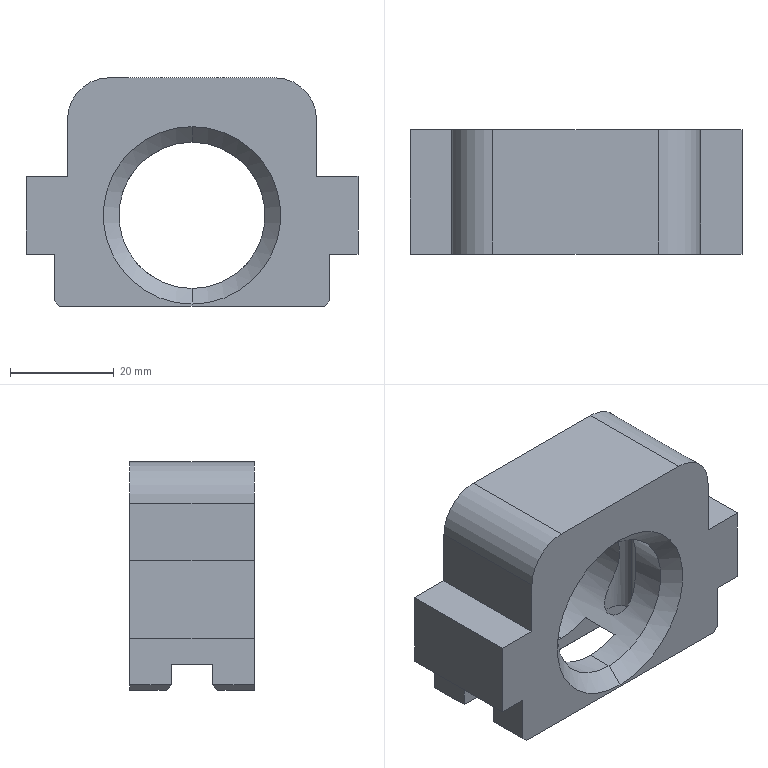Part | SolidWorks | features ICE 3, Chamfer 2, Extrusion 1 | 1 solid | 37 faces | box 64 x 24 x 44 mm | volume 38268 mm3 | plane 27 | cylinder 8 | cone 2 | commonest cylinder face diameters 6 x4 16 x2 28.2 x2
STEP:
#1=CARTESIAN_POINT('',(0.,3.,-12.4));
#2=VERTEX_POINT('',#1);
#3=CARTESIAN_POINT('',(0.,3.,-40.6));
#4=VERTEX_POINT('',#3);
#5=CARTESIAN_POINT('',(0.,3.,-26.5));
#6=DIRECTION('',(0.,-1.,0.));
#7=DIRECTION('',(0.,0.,1.));
#8=AXIS2_PLACEMENT_3D('',#5,#6,#7);
#9=CIRCLE('',#8,14.1);
#10=EDGE_CURVE('',#2,#4,#9,.T.);
#11=ORIENTED_EDGE('',*,*,#10,.F.);
#12=CARTESIAN_POINT('',(0.,0.,-9.4));
#13=VERTEX_POINT('',#12);
#14=CARTESIAN_POINT('',(0.,3.,-12.4));
#15=DIRECTION('',(0.,-0.7071,0.7071));
#16=VECTOR('',#15,1000.);
#17=LINE('',#14,#16);
#18=EDGE_CURVE('',#2,#13,#17,.T.);
#19=ORIENTED_EDGE('',*,*,#18,.T.);
#20=CARTESIAN_POINT('',(0.,0.,-43.6));
#21=VERTEX_POINT('',#20);
#22=CARTESIAN_POINT('',(0.,0.,-26.5));
#23=DIRECTION('',(0.,1.,0.));
#24=DIRECTION('',(0.,0.,1.));
#25=AXIS2_PLACEMENT_3D('',#22,#23,#24);
#26=CIRCLE('',#25,17.1);
#27=EDGE_CURVE('',#21,#13,#26,.T.);
#28=ORIENTED_EDGE('',*,*,#27,.F.);
#29=CARTESIAN_POINT('',(0.,3.,-40.6));
#30=DIRECTION('',(0.,-0.7071,-0.7071));
#31=VECTOR('',#30,1000.);
#32=LINE('',#29,#31);
#33=EDGE_CURVE('',#4,#21,#32,.T.);
#34=ORIENTED_EDGE('',*,*,#33,.F.);
#35=EDGE_LOOP('',(#11,#19,#28,#34));
#36=FACE_OUTER_BOUND('',#35,.T.);
#37=CARTESIAN_POINT('',(0.,3.,-26.5));
#38=DIRECTION('',(0.,-1.,0.));
#39=DIRECTION('',(0.,0.,-1.));
#40=AXIS2_PLACEMENT_3D('',#37,#38,#39);
#41=CONICAL_SURFACE('',#40,14.1,0.7854);
#42=ADVANCED_FACE('',(#36),#41,.F.);
#43=CARTESIAN_POINT('',(-9.,12.,-15.646));
#44=VERTEX_POINT('',#43);
#45=CARTESIAN_POINT('',(-9.,12.,-37.354));
#46=VERTEX_POINT('',#45);
#47=CARTESIAN_POINT('',(-9.,12.,-15.646));
#48=CARTESIAN_POINT('',(-9.,11.703,-15.646));
#49=CARTESIAN_POINT('',(-9.044,11.415,-15.682));
#50=CARTESIAN_POINT('',(-9.167,11.003,-15.787));
#51=CARTESIAN_POINT('',(-9.217,10.872,-15.829));
#52=CARTESIAN_POINT('',(-9.332,10.622,-15.93));
#53=CARTESIAN_POINT('',(-9.397,10.502,-15.988));
#54=CARTESIAN_POINT('',(-9.61,10.167,-16.181));
#55=CARTESIAN_POINT('',(-9.774,9.975,-16.335));
#56=CARTESIAN_POINT('',(-10.121,9.649,-16.68));
#57=CARTESIAN_POINT('',(-10.301,9.518,-16.868));
#58=CARTESIAN_POINT('',(-10.665,9.305,-17.273));
#59=CARTESIAN_POINT('',(-10.849,9.223,-17.49));
#60=CARTESIAN_POINT('',(-11.204,9.101,-17.935));
#61=CARTESIAN_POINT('',(-11.377,9.061,-18.165));
#62=CARTESIAN_POINT('',(-11.71,9.009,-18.64));
#63=CARTESIAN_POINT('',(-11.871,8.999,-18.886));
#64=CARTESIAN_POINT('',(-12.176,9.001,-19.384));
#65=CARTESIAN_POINT('',(-12.32,9.014,-19.636));
#66=CARTESIAN_POINT('',(-12.726,9.076,-20.402));
#67=CARTESIAN_POINT('',(-12.964,9.15,-20.925));
#68=CARTESIAN_POINT('',(-13.375,9.324,-22.));
#69=CARTESIAN_POINT('',(-13.548,9.425,-22.55));
#70=CARTESIAN_POINT('',(-13.823,9.612,-23.661));
#71=CARTESIAN_POINT('',(-13.927,9.699,-24.225));
#72=CARTESIAN_POINT('',(-14.067,9.823,-25.372));
#73=CARTESIAN_POINT('',(-14.101,9.859,-25.96));
#74=CARTESIAN_POINT('',(-14.098,9.856,-27.112));
#75=CARTESIAN_POINT('',(-14.062,9.819,-27.683));
#76=CARTESIAN_POINT('',(-13.92,9.693,-28.814));
#77=CARTESIAN_POINT('',(-13.816,9.606,-29.375));
#78=CARTESIAN_POINT('',(-13.396,9.324,-31.046));
#79=CARTESIAN_POINT('',(-12.988,9.114,-32.109));
#80=CARTESIAN_POINT('',(-12.307,9.013,-33.387));
#81=CARTESIAN_POINT('',(-12.161,9.,-33.641));
#82=CARTESIAN_POINT('',(-11.856,9.,-34.137));
#83=CARTESIAN_POINT('',(-11.696,9.011,-34.38));
#84=CARTESIAN_POINT('',(-11.362,9.064,-34.854));
#85=CARTESIAN_POINT('',(-11.187,9.106,-35.087));
#86=CARTESIAN_POINT('',(-10.833,9.23,-35.53));
#87=CARTESIAN_POINT('',(-10.653,9.311,-35.741));
#88=CARTESIAN_POINT('',(-10.293,9.524,-36.14));
#89=CARTESIAN_POINT('',(-10.11,9.658,-36.331));
#90=CARTESIAN_POINT('',(-9.852,9.902,-36.587));
#91=CARTESIAN_POINT('',(-9.769,9.99,-36.668));
#92=CARTESIAN_POINT('',(-9.61,10.183,-36.819));
#93=CARTESIAN_POINT('',(-9.533,10.288,-36.89));
#94=CARTESIAN_POINT('',(-9.322,10.622,-37.08));
#95=CARTESIAN_POINT('',(-9.207,10.869,-37.18));
#96=CARTESIAN_POINT('',(-9.043,11.419,-37.319));
#97=CARTESIAN_POINT('',(-9.,11.705,-37.354));
#98=CARTESIAN_POINT('',(-9.,12.,-37.354));
#99=B_SPLINE_CURVE_WITH_KNOTS('',3,(#47,#48,#49,#50,#51,#52,#53,#54,#55,#56,#57,#58,#59,#60,#61,#62,#63,#64,#65,#66,#67,#68,#69,#70,#71,#72,#73,#74,#75,#76,#77,#78,#79,#80,#81,#82,#83,#84,#85,#86,#87,#88,#89,#90,#91,#92,#93,#94,#95,#96,#97,#98),.UNSPECIFIED.,.F.,.F.,(4,2,2,2,2,2,2,2,2,2,2,2,2,2,2,2,2,2,2,2,2,2,2,2,2,4),(0.,0.0008757,0.001313,0.001751,0.002627,0.003503,0.004378,0.005254,0.00613,0.007005,0.008757,0.01051,0.01226,0.01401,0.01576,0.01751,0.02102,0.02189,0.02277,0.02364,0.02452,0.02539,0.02583,0.02627,0.02715,0.02802),.UNSPECIFIED.);
#100=EDGE_CURVE('',#44,#46,#99,.T.);
#101=ORIENTED_EDGE('',*,*,#100,.F.);
#102=CARTESIAN_POINT('',(-9.,12.,-37.354));
#103=CARTESIAN_POINT('',(-9.,12.295,-37.354));
#104=CARTESIAN_POINT('',(-9.044,12.585,-37.318));
#105=CARTESIAN_POINT('',(-9.167,12.997,-37.214));
#106=CARTESIAN_POINT('',(-9.217,13.128,-37.171));
#107=CARTESIAN_POINT('',(-9.331,13.377,-37.071));
#108=CARTESIAN_POINT('',(-9.397,13.497,-37.013));
#109=CARTESIAN_POINT('',(-9.609,13.832,-36.82));
#110=CARTESIAN_POINT('',(-9.773,14.024,-36.667));
#111=CARTESIAN_POINT('',(-10.119,14.349,-36.322));
#112=CARTESIAN_POINT('',(-10.298,14.48,-36.135));
#113=CARTESIAN_POINT('',(-10.662,14.693,-35.731));
#114=CARTESIAN_POINT('',(-10.846,14.775,-35.514));
#115=CARTESIAN_POINT('',(-11.2,14.897,-35.07));
#116=CARTESIAN_POINT('',(-11.372,14.938,-34.841));
#117=CARTESIAN_POINT('',(-11.705,14.99,-34.367));
#118=CARTESIAN_POINT('',(-11.867,15.001,-34.121));
#119=CARTESIAN_POINT('',(-12.171,14.999,-33.625));
#120=CARTESIAN_POINT('',(-12.315,14.987,-33.373));
#121=CARTESIAN_POINT('',(-12.721,14.925,-32.609));
#122=CARTESIAN_POINT('',(-12.959,14.851,-32.087));
#123=CARTESIAN_POINT('',(-13.37,14.678,-31.014));
#124=CARTESIAN_POINT('',(-13.543,14.578,-30.465));
#125=CARTESIAN_POINT('',(-13.819,14.392,-29.359));
#126=CARTESIAN_POINT('',(-13.923,14.305,-28.8));
#127=CARTESIAN_POINT('',(-14.029,14.211,-27.946));
#128=CARTESIAN_POINT('',(-14.055,14.186,-27.66));
#129=CARTESIAN_POINT('',(-14.091,14.151,-27.081));
#130=CARTESIAN_POINT('',(-14.1,14.142,-26.787));
#131=CARTESIAN_POINT('',(-14.1,14.143,-25.912));
#132=CARTESIAN_POINT('',(-14.064,14.18,-25.337));
#133=CARTESIAN_POINT('',(-13.923,14.304,-24.202));
#134=CARTESIAN_POINT('',(-13.819,14.391,-23.642));
#135=CARTESIAN_POINT('',(-13.542,14.579,-22.532));
#136=CARTESIAN_POINT('',(-13.369,14.679,-21.982));
#137=CARTESIAN_POINT('',(-12.959,14.851,-20.915));
#138=CARTESIAN_POINT('',(-12.723,14.924,-20.395));
#139=CARTESIAN_POINT('',(-12.318,14.986,-19.632));
#140=CARTESIAN_POINT('',(-12.175,14.999,-19.381));
#141=CARTESIAN_POINT('',(-11.87,15.001,-18.885));
#142=CARTESIAN_POINT('',(-11.709,14.991,-18.638));
#143=CARTESIAN_POINT('',(-11.374,14.939,-18.162));
#144=CARTESIAN_POINT('',(-11.201,14.898,-17.931));
#145=CARTESIAN_POINT('',(-10.844,14.775,-17.483));
#146=CARTESIAN_POINT('',(-10.661,14.693,-17.268));
#147=CARTESIAN_POINT('',(-10.299,14.48,-16.866));
#148=CARTESIAN_POINT('',(-10.119,14.35,-16.678));
#149=CARTESIAN_POINT('',(-9.771,14.022,-16.332));
#150=CARTESIAN_POINT('',(-9.61,13.832,-16.18));
#151=CARTESIAN_POINT('',(-9.397,13.497,-15.987));
#152=CARTESIAN_POINT('',(-9.331,13.377,-15.929));
#153=CARTESIAN_POINT('',(-9.217,13.129,-15.829));
#154=CARTESIAN_POINT('',(-9.168,12.999,-15.787));
#155=CARTESIAN_POINT('',(-9.086,12.727,-15.718));
#156=CARTESIAN_POINT('',(-9.054,12.584,-15.691));
#157=CARTESIAN_POINT('',(-9.011,12.295,-15.655));
#158=CARTESIAN_POINT('',(-9.,12.148,-15.646));
#159=CARTESIAN_POINT('',(-9.,12.,-15.646));
#160=B_SPLINE_CURVE_WITH_KNOTS('',3,(#102,#103,#104,#105,#106,#107,#108,#109,#110,#111,#112,#113,#114,#115,#116,#117,#118,#119,#120,#121,#122,#123,#124,#125,#126,#127,#128,#129,#130,#131,#132,#133,#134,#135,#136,#137,#138,#139,#140,#141,#142,#143,#144,#145,#146,#147,#148,#149,#150,#151,#152,#153,#154,#155,#156,#157,#158,#159),.UNSPECIFIED.,.F.,.F.,(4,2,2,2,2,2,2,2,2,2,2,2,2,2,2,2,2,2,2,2,2,2,2,2,2,2,2,2,4),(0.02802,0.0289,0.02933,0.02977,0.03065,0.03152,0.0324,0.03327,0.03415,0.03502,0.03677,0.03853,0.04028,0.04115,0.04203,0.04378,0.04553,0.04728,0.04903,0.04991,0.05078,0.05166,0.05253,0.05341,0.05428,0.05472,0.05516,0.05559,0.05603),.UNSPECIFIED.);
#161=EDGE_CURVE('',#46,#44,#160,.T.);
#162=ORIENTED_EDGE('',*,*,#161,.F.);
#163=EDGE_LOOP('',(#101,#162));
#164=FACE_BOUND('',#163,.T.);
#165=CARTESIAN_POINT('',(0.,24.,-40.6));
#166=VERTEX_POINT('',#165);
#167=CARTESIAN_POINT('',(0.,24.,-12.4));
#168=VERTEX_POINT('',#167);
#169=CARTESIAN_POINT('',(0.,24.,-26.5));
#170=DIRECTION('',(0.,1.,0.));
#171=DIRECTION('',(0.,0.,1.));
#172=AXIS2_PLACEMENT_3D('',#169,#170,#171);
#173=CIRCLE('',#172,14.1);
#174=EDGE_CURVE('',#166,#168,#173,.T.);
#175=ORIENTED_EDGE('',*,*,#174,.T.);
#176=CARTESIAN_POINT('',(0.,35.,-12.4));
#177=DIRECTION('',(0.,-1.,0.));
#178=VECTOR('',#177,1000.);
#179=LINE('',#176,#178);
#180=EDGE_CURVE('',#168,#2,#179,.T.);
#181=ORIENTED_EDGE('',*,*,#180,.T.);
#182=ORIENTED_EDGE('',*,*,#10,.T.);
#183=CARTESIAN_POINT('',(0.,8.,-40.6));
#184=VERTEX_POINT('',#183);
#185=CARTESIAN_POINT('',(0.,35.,-40.6));
#186=DIRECTION('',(0.,-1.,0.));
#187=VECTOR('',#186,1000.);
#188=LINE('',#185,#187);
#189=EDGE_CURVE('',#184,#4,#188,.T.);
#190=ORIENTED_EDGE('',*,*,#189,.F.);
#191=CARTESIAN_POINT('',(-6.524,8.,-39.));
#192=VERTEX_POINT('',#191);
#193=CARTESIAN_POINT('',(0.,8.,-26.5));
#194=DIRECTION('',(0.,-1.,0.));
#195=DIRECTION('',(0.,0.,-1.));
#196=AXIS2_PLACEMENT_3D('',#193,#194,#195);
#197=CIRCLE('',#196,14.1);
#198=EDGE_CURVE('',#192,#184,#197,.T.);
#199=ORIENTED_EDGE('',*,*,#198,.F.);
#200=CARTESIAN_POINT('',(-6.524,16.,-39.));
#201=VERTEX_POINT('',#200);
#202=CARTESIAN_POINT('',(-6.524,35.,-39.));
#203=DIRECTION('',(0.,-1.,0.));
#204=VECTOR('',#203,1000.);
#205=LINE('',#202,#204);
#206=EDGE_CURVE('',#201,#192,#205,.T.);
#207=ORIENTED_EDGE('',*,*,#206,.F.);
#208=CARTESIAN_POINT('',(0.,16.,-40.6));
#209=VERTEX_POINT('',#208);
#210=CARTESIAN_POINT('',(0.,16.,-26.5));
#211=DIRECTION('',(0.,1.,0.));
#212=DIRECTION('',(0.,0.,1.));
#213=AXIS2_PLACEMENT_3D('',#210,#211,#212);
#214=CIRCLE('',#213,14.1);
#215=EDGE_CURVE('',#209,#201,#214,.T.);
#216=ORIENTED_EDGE('',*,*,#215,.F.);
#217=CARTESIAN_POINT('',(0.,35.,-40.6));
#218=DIRECTION('',(0.,-1.,0.));
#219=VECTOR('',#218,1000.);
#220=LINE('',#217,#219);
#221=EDGE_CURVE('',#166,#209,#220,.T.);
#222=ORIENTED_EDGE('',*,*,#221,.F.);
#223=EDGE_LOOP('',(#175,#181,#182,#190,#199,#207,#216,#222));
#224=FACE_OUTER_BOUND('',#223,.T.);
#225=CARTESIAN_POINT('',(0.,35.,-26.5));
#226=DIRECTION('',(0.,-1.,0.));
#227=DIRECTION('',(0.,0.,-1.));
#228=AXIS2_PLACEMENT_3D('',#225,#226,#227);
#229=CYLINDRICAL_SURFACE('',#228,14.1);
#230=ADVANCED_FACE('',(#164,#224),#229,.F.);
#231=CARTESIAN_POINT('',(15.,12.,-4.));
#232=VERTEX_POINT('',#231);
#233=CARTESIAN_POINT('',(9.,12.,-4.));
#234=VERTEX_POINT('',#233);
#235=CARTESIAN_POINT('',(12.,12.,-4.));
#236=DIRECTION('',(0.,0.,-1.));
#237=DIRECTION('',(-1.,0.,0.));
#238=AXIS2_PLACEMENT_3D('',#235,#236,#237);
#239=CIRCLE('',#238,3.);
#240=EDGE_CURVE('',#232,#234,#239,.T.);
#241=ORIENTED_EDGE('',*,*,#240,.F.);
#242=CARTESIAN_POINT('',(15.,12.,-39.));
#243=VERTEX_POINT('',#242);
#244=CARTESIAN_POINT('',(15.,12.,-4.));
#245=DIRECTION('',(0.,0.,-1.));
#246=VECTOR('',#245,1000.);
#247=LINE('',#244,#246);
#248=EDGE_CURVE('',#232,#243,#247,.T.);
#249=ORIENTED_EDGE('',*,*,#248,.T.);
#250=CARTESIAN_POINT('',(9.,12.,-39.));
#251=VERTEX_POINT('',#250);
#252=CARTESIAN_POINT('',(12.,12.,-39.));
#253=DIRECTION('',(0.,0.,-1.));
#254=DIRECTION('',(-1.,0.,0.));
#255=AXIS2_PLACEMENT_3D('',#252,#253,#254);
#256=CIRCLE('',#255,3.);
#257=EDGE_CURVE('',#243,#251,#256,.T.);
#258=ORIENTED_EDGE('',*,*,#257,.T.);
#259=CARTESIAN_POINT('',(9.,12.,-37.354));
#260=VERTEX_POINT('',#259);
#261=CARTESIAN_POINT('',(9.,12.,-4.));
#262=DIRECTION('',(0.,0.,-1.));
#263=VECTOR('',#262,1000.);
#264=LINE('',#261,#263);
#265=EDGE_CURVE('',#260,#251,#264,.T.);
#266=ORIENTED_EDGE('',*,*,#265,.F.);
#267=CARTESIAN_POINT('',(9.,12.,-15.646));
#268=VERTEX_POINT('',#267);
#269=CARTESIAN_POINT('',(9.,12.,-37.354));
#270=CARTESIAN_POINT('',(9.,11.705,-37.354));
#271=CARTESIAN_POINT('',(9.044,11.415,-37.318));
#272=CARTESIAN_POINT('',(9.167,11.003,-37.214));
#273=CARTESIAN_POINT('',(9.217,10.872,-37.171));
#274=CARTESIAN_POINT('',(9.331,10.623,-37.071));
#275=CARTESIAN_POINT('',(9.397,10.503,-37.013));
#276=CARTESIAN_POINT('',(9.609,10.168,-36.82));
#277=CARTESIAN_POINT('',(9.773,9.976,-36.667));
#278=CARTESIAN_POINT('',(10.119,9.651,-36.322));
#279=CARTESIAN_POINT('',(10.298,9.52,-36.135));
#280=CARTESIAN_POINT('',(10.662,9.307,-35.731));
#281=CARTESIAN_POINT('',(10.846,9.225,-35.514));
#282=CARTESIAN_POINT('',(11.2,9.103,-35.07));
#283=CARTESIAN_POINT('',(11.372,9.062,-34.841));
#284=CARTESIAN_POINT('',(11.705,9.01,-34.367));
#285=CARTESIAN_POINT('',(11.867,8.999,-34.121));
#286=CARTESIAN_POINT('',(12.171,9.001,-33.625));
#287=CARTESIAN_POINT('',(12.315,9.013,-33.373));
#288=CARTESIAN_POINT('',(12.721,9.075,-32.609));
#289=CARTESIAN_POINT('',(12.959,9.149,-32.087));
#290=CARTESIAN_POINT('',(13.37,9.322,-31.014));
#291=CARTESIAN_POINT('',(13.543,9.422,-30.465));
#292=CARTESIAN_POINT('',(13.819,9.608,-29.359));
#293=CARTESIAN_POINT('',(13.923,9.695,-28.8));
#294=CARTESIAN_POINT('',(14.029,9.789,-27.946));
#295=CARTESIAN_POINT('',(14.055,9.814,-27.66));
#296=CARTESIAN_POINT('',(14.091,9.849,-27.081));
#297=CARTESIAN_POINT('',(14.1,9.858,-26.787));
#298=CARTESIAN_POINT('',(14.1,9.857,-25.912));
#299=CARTESIAN_POINT('',(14.064,9.82,-25.337));
#300=CARTESIAN_POINT('',(13.923,9.696,-24.202));
#301=CARTESIAN_POINT('',(13.819,9.609,-23.642));
#302=CARTESIAN_POINT('',(13.542,9.421,-22.532));
#303=CARTESIAN_POINT('',(13.369,9.321,-21.982));
#304=CARTESIAN_POINT('',(12.959,9.149,-20.915));
#305=CARTESIAN_POINT('',(12.723,9.076,-20.395));
#306=CARTESIAN_POINT('',(12.318,9.014,-19.632));
#307=CARTESIAN_POINT('',(12.175,9.001,-19.381));
#308=CARTESIAN_POINT('',(11.87,8.999,-18.885));
#309=CARTESIAN_POINT('',(11.709,9.009,-18.638));
#310=CARTESIAN_POINT('',(11.374,9.061,-18.162));
#311=CARTESIAN_POINT('',(11.201,9.102,-17.931));
#312=CARTESIAN_POINT('',(10.844,9.225,-17.483));
#313=CARTESIAN_POINT('',(10.661,9.307,-17.268));
#314=CARTESIAN_POINT('',(10.299,9.52,-16.866));
#315=CARTESIAN_POINT('',(10.119,9.65,-16.678));
#316=CARTESIAN_POINT('',(9.771,9.978,-16.332));
#317=CARTESIAN_POINT('',(9.61,10.168,-16.18));
#318=CARTESIAN_POINT('',(9.397,10.503,-15.987));
#319=CARTESIAN_POINT('',(9.331,10.623,-15.929));
#320=CARTESIAN_POINT('',(9.217,10.871,-15.829));
#321=CARTESIAN_POINT('',(9.168,11.001,-15.787));
#322=CARTESIAN_POINT('',(9.086,11.273,-15.718));
#323=CARTESIAN_POINT('',(9.054,11.416,-15.691));
#324=CARTESIAN_POINT('',(9.011,11.705,-15.655));
#325=CARTESIAN_POINT('',(9.,11.852,-15.646));
#326=CARTESIAN_POINT('',(9.,12.,-15.646));
#327=B_SPLINE_CURVE_WITH_KNOTS('',3,(#269,#270,#271,#272,#273,#274,#275,#276,#277,#278,#279,#280,#281,#282,#283,#284,#285,#286,#287,#288,#289,#290,#291,#292,#293,#294,#295,#296,#297,#298,#299,#300,#301,#302,#303,#304,#305,#306,#307,#308,#309,#310,#311,#312,#313,#314,#315,#316,#317,#318,#319,#320,#321,#322,#323,#324,#325,#326),.UNSPECIFIED.,.F.,.F.,(4,2,2,2,2,2,2,2,2,2,2,2,2,2,2,2,2,2,2,2,2,2,2,2,2,2,2,2,4),(0.02802,0.0289,0.02933,0.02977,0.03065,0.03152,0.0324,0.03327,0.03415,0.03502,0.03677,0.03853,0.04028,0.04115,0.04203,0.04378,0.04553,0.04728,0.04903,0.04991,0.05078,0.05166,0.05253,0.05341,0.05428,0.05472,0.05516,0.05559,0.05603),.UNSPECIFIED.);
#328=EDGE_CURVE('',#260,#268,#327,.T.);
#329=ORIENTED_EDGE('',*,*,#328,.T.);
#330=CARTESIAN_POINT('',(9.,12.,-4.));
#331=DIRECTION('',(0.,0.,-1.));
#332=VECTOR('',#331,1000.);
#333=LINE('',#330,#332);
#334=EDGE_CURVE('',#234,#268,#333,.T.);
#335=ORIENTED_EDGE('',*,*,#334,.F.);
#336=EDGE_LOOP('',(#241,#249,#258,#266,#329,#335));
#337=FACE_OUTER_BOUND('',#336,.T.);
#338=CARTESIAN_POINT('',(12.,12.,-4.));
#339=DIRECTION('',(0.,0.,-1.));
#340=DIRECTION('',(-1.,0.,0.));
#341=AXIS2_PLACEMENT_3D('',#338,#339,#340);
#342=CYLINDRICAL_SURFACE('',#341,3.);
#343=ADVANCED_FACE('',(#337),#342,.F.);
#344=CARTESIAN_POINT('',(-9.,12.,-4.));
#345=VERTEX_POINT('',#344);
#346=CARTESIAN_POINT('',(-15.,12.,-4.));
#347=VERTEX_POINT('',#346);
#348=CARTESIAN_POINT('',(-12.,12.,-4.));
#349=DIRECTION('',(0.,0.,-1.));
#350=DIRECTION('',(1.,0.,0.));
#351=AXIS2_PLACEMENT_3D('',#348,#349,#350);
#352=CIRCLE('',#351,3.);
#353=EDGE_CURVE('',#345,#347,#352,.T.);
#354=ORIENTED_EDGE('',*,*,#353,.F.);
#355=CARTESIAN_POINT('',(-9.,12.,-4.));
#356=DIRECTION('',(0.,0.,-1.));
#357=VECTOR('',#356,1000.);
#358=LINE('',#355,#357);
#359=EDGE_CURVE('',#345,#44,#358,.T.);
#360=ORIENTED_EDGE('',*,*,#359,.T.);
#361=ORIENTED_EDGE('',*,*,#100,.T.);
#362=CARTESIAN_POINT('',(-9.,12.,-39.));
#363=VERTEX_POINT('',#362);
#364=CARTESIAN_POINT('',(-9.,12.,-4.));
#365=DIRECTION('',(0.,0.,-1.));
#366=VECTOR('',#365,1000.);
#367=LINE('',#364,#366);
#368=EDGE_CURVE('',#46,#363,#367,.T.);
#369=ORIENTED_EDGE('',*,*,#368,.T.);
#370=CARTESIAN_POINT('',(-15.,12.,-39.));
#371=VERTEX_POINT('',#370);
#372=CARTESIAN_POINT('',(-12.,12.,-39.));
#373=DIRECTION('',(0.,0.,-1.));
#374=DIRECTION('',(1.,0.,0.));
#375=AXIS2_PLACEMENT_3D('',#372,#373,#374);
#376=CIRCLE('',#375,3.);
#377=EDGE_CURVE('',#363,#371,#376,.T.);
#378=ORIENTED_EDGE('',*,*,#377,.T.);
#379=CARTESIAN_POINT('',(-15.,12.,-4.));
#380=DIRECTION('',(0.,0.,-1.));
#381=VECTOR('',#380,1000.);
#382=LINE('',#379,#381);
#383=EDGE_CURVE('',#347,#371,#382,.T.);
#384=ORIENTED_EDGE('',*,*,#383,.F.);
#385=EDGE_LOOP('',(#354,#360,#361,#369,#378,#384));
#386=FACE_OUTER_BOUND('',#385,.T.);
#387=CARTESIAN_POINT('',(-12.,12.,-4.));
#388=DIRECTION('',(0.,0.,-1.));
#389=DIRECTION('',(-1.,0.,0.));
#390=AXIS2_PLACEMENT_3D('',#387,#388,#389);
#391=CYLINDRICAL_SURFACE('',#390,3.);
#392=ADVANCED_FACE('',(#386),#391,.F.);
#393=CARTESIAN_POINT('',(-12.,12.,-39.));
#394=DIRECTION('',(0.,0.,-1.));
#395=DIRECTION('',(1.,0.,0.));
#396=AXIS2_PLACEMENT_3D('',#393,#394,#395);
#397=CIRCLE('',#396,3.);
#398=EDGE_CURVE('',#371,#363,#397,.T.);
#399=ORIENTED_EDGE('',*,*,#398,.F.);
#400=ORIENTED_EDGE('',*,*,#377,.F.);
#401=EDGE_LOOP('',(#399,#400));
#402=FACE_BOUND('',#401,.T.);
#403=CARTESIAN_POINT('',(-26.5,16.,-39.));
#404=VERTEX_POINT('',#403);
#405=CARTESIAN_POINT('',(37.5,16.,-39.));
#406=DIRECTION('',(-1.,0.,0.));
#407=VECTOR('',#406,1000.);
#408=LINE('',#405,#407);
#409=EDGE_CURVE('',#201,#404,#408,.T.);
#410=ORIENTED_EDGE('',*,*,#409,.F.);
#411=ORIENTED_EDGE('',*,*,#206,.T.);
#412=CARTESIAN_POINT('',(-26.5,8.,-39.));
#413=VERTEX_POINT('',#412);
#414=CARTESIAN_POINT('',(37.5,8.,-39.));
#415=DIRECTION('',(-1.,0.,0.));
#416=VECTOR('',#415,1000.);
#417=LINE('',#414,#416);
#418=EDGE_CURVE('',#192,#413,#417,.T.);
#419=ORIENTED_EDGE('',*,*,#418,.T.);
#420=CARTESIAN_POINT('',(-26.5,16.,-39.));
#421=DIRECTION('',(0.,1.,0.));
#422=VECTOR('',#421,1000.);
#423=LINE('',#420,#422);
#424=EDGE_CURVE('',#413,#404,#423,.T.);
#425=ORIENTED_EDGE('',*,*,#424,.T.);
#426=EDGE_LOOP('',(#410,#411,#419,#425));
#427=FACE_OUTER_BOUND('',#426,.T.);
#428=CARTESIAN_POINT('',(37.5,16.,-39.));
#429=DIRECTION('',(0.,0.,1.));
#430=DIRECTION('',(1.,0.,0.));
#431=AXIS2_PLACEMENT_3D('',#428,#429,#430);
#432=PLANE('',#431);
#433=ADVANCED_FACE('',(#402,#427),#432,.F.);
#434=CARTESIAN_POINT('',(-25.5,7.,-44.));
#435=VERTEX_POINT('',#434);
#436=CARTESIAN_POINT('',(25.5,7.,-44.));
#437=VERTEX_POINT('',#436);
#438=CARTESIAN_POINT('',(-26.5,7.,-44.));
#439=DIRECTION('',(1.,0.,0.));
#440=VECTOR('',#439,1000.);
#441=LINE('',#438,#440);
#442=EDGE_CURVE('',#435,#437,#441,.T.);
#443=ORIENTED_EDGE('',*,*,#442,.T.);
#444=CARTESIAN_POINT('',(25.5,0.,-44.));
#445=VERTEX_POINT('',#444);
#446=CARTESIAN_POINT('',(25.5,24.,-44.));
#447=DIRECTION('',(0.,-1.,0.));
#448=VECTOR('',#447,1000.);
#449=LINE('',#446,#448);
#450=EDGE_CURVE('',#437,#445,#449,.T.);
#451=ORIENTED_EDGE('',*,*,#450,.T.);
#452=CARTESIAN_POINT('',(-25.5,0.,-44.));
#453=VERTEX_POINT('',#452);
#454=CARTESIAN_POINT('',(-26.5,0.,-44.));
#455=DIRECTION('',(-1.,0.,0.));
#456=VECTOR('',#455,1000.);
#457=LINE('',#454,#456);
#458=EDGE_CURVE('',#445,#453,#457,.T.);
#459=ORIENTED_EDGE('',*,*,#458,.T.);
#460=CARTESIAN_POINT('',(-25.5,24.,-44.));
#461=DIRECTION('',(0.,1.,0.));
#462=VECTOR('',#461,1000.);
#463=LINE('',#460,#462);
#464=EDGE_CURVE('',#453,#435,#463,.T.);
#465=ORIENTED_EDGE('',*,*,#464,.T.);
#466=EDGE_LOOP('',(#443,#451,#459,#465));
#467=FACE_OUTER_BOUND('',#466,.T.);
#468=CARTESIAN_POINT('',(-26.5,24.,-44.));
#469=DIRECTION('',(0.,0.,1.));
#470=DIRECTION('',(1.,0.,0.));
#471=AXIS2_PLACEMENT_3D('',#468,#469,#470);
#472=PLANE('',#471);
#473=ADVANCED_FACE('',(#467),#472,.F.);
#474=CARTESIAN_POINT('',(-24.,0.,-8.));
#475=VERTEX_POINT('',#474);
#476=CARTESIAN_POINT('',(-16.,0.,0.));
#477=VERTEX_POINT('',#476);
#478=CARTESIAN_POINT('',(-16.,0.,-8.));
#479=DIRECTION('',(0.,1.,0.));
#480=DIRECTION('',(0.,0.,1.));
#481=AXIS2_PLACEMENT_3D('',#478,#479,#480);
#482=CIRCLE('',#481,8.);
#483=EDGE_CURVE('',#475,#477,#482,.T.);
#484=ORIENTED_EDGE('',*,*,#483,.T.);
#485=CARTESIAN_POINT('',(-16.,24.,0.));
#486=VERTEX_POINT('',#485);
#487=CARTESIAN_POINT('',(-16.,24.,0.));
#488=DIRECTION('',(0.,-1.,0.));
#489=VECTOR('',#488,1000.);
#490=LINE('',#487,#489);
#491=EDGE_CURVE('',#486,#477,#490,.T.);
#492=ORIENTED_EDGE('',*,*,#491,.F.);
#493=CARTESIAN_POINT('',(-24.,24.,-8.));
#494=VERTEX_POINT('',#493);
#495=CARTESIAN_POINT('',(-16.,24.,-8.));
#496=DIRECTION('',(0.,1.,0.));
#497=DIRECTION('',(0.,0.,1.));
#498=AXIS2_PLACEMENT_3D('',#495,#496,#497);
#499=CIRCLE('',#498,8.);
#500=EDGE_CURVE('',#494,#486,#499,.T.);
#501=ORIENTED_EDGE('',*,*,#500,.F.);
#502=CARTESIAN_POINT('',(-24.,24.,-8.));
#503=DIRECTION('',(0.,-1.,0.));
#504=VECTOR('',#503,1000.);
#505=LINE('',#502,#504);
#506=EDGE_CURVE('',#494,#475,#505,.T.);
#507=ORIENTED_EDGE('',*,*,#506,.T.);
#508=EDGE_LOOP('',(#484,#492,#501,#507));
#509=FACE_OUTER_BOUND('',#508,.T.);
#510=CARTESIAN_POINT('',(-16.,24.,-8.));
#511=DIRECTION('',(0.,-1.,0.));
#512=DIRECTION('',(0.,0.,-1.));
#513=AXIS2_PLACEMENT_3D('',#510,#511,#512);
#514=CYLINDRICAL_SURFACE('',#513,8.);
#515=ADVANCED_FACE('',(#509),#514,.T.);
#516=CARTESIAN_POINT('',(16.,0.,0.));
#517=VERTEX_POINT('',#516);
#518=CARTESIAN_POINT('',(-16.,0.,0.));
#519=DIRECTION('',(1.,0.,0.));
#520=VECTOR('',#519,1000.);
#521=LINE('',#518,#520);
#522=EDGE_CURVE('',#477,#517,#521,.T.);
#523=ORIENTED_EDGE('',*,*,#522,.T.);
#524=CARTESIAN_POINT('',(16.,24.,0.));
#525=VERTEX_POINT('',#524);
#526=CARTESIAN_POINT('',(16.,24.,0.));
#527=DIRECTION('',(0.,-1.,0.));
#528=VECTOR('',#527,1000.);
#529=LINE('',#526,#528);
#530=EDGE_CURVE('',#525,#517,#529,.T.);
#531=ORIENTED_EDGE('',*,*,#530,.F.);
#532=CARTESIAN_POINT('',(-16.,24.,0.));
#533=DIRECTION('',(1.,0.,0.));
#534=VECTOR('',#533,1000.);
#535=LINE('',#532,#534);
#536=EDGE_CURVE('',#486,#525,#535,.T.);
#537=ORIENTED_EDGE('',*,*,#536,.F.);
#538=ORIENTED_EDGE('',*,*,#491,.T.);
#539=EDGE_LOOP('',(#523,#531,#537,#538));
#540=FACE_OUTER_BOUND('',#539,.T.);
#541=CARTESIAN_POINT('',(-16.,24.,0.));
#542=DIRECTION('',(0.,0.,-1.));
#543=DIRECTION('',(-1.,0.,0.));
#544=AXIS2_PLACEMENT_3D('',#541,#542,#543);
#545=PLANE('',#544);
#546=ADVANCED_FACE('',(#540),#545,.F.);
#547=CARTESIAN_POINT('',(24.,0.,-8.));
#548=VERTEX_POINT('',#547);
#549=CARTESIAN_POINT('',(16.,0.,-8.));
#550=DIRECTION('',(0.,1.,0.));
#551=DIRECTION('',(0.,0.,-1.));
#552=AXIS2_PLACEMENT_3D('',#549,#550,#551);
#553=CIRCLE('',#552,8.);
#554=EDGE_CURVE('',#517,#548,#553,.T.);
#555=ORIENTED_EDGE('',*,*,#554,.T.);
#556=CARTESIAN_POINT('',(24.,24.,-8.));
#557=VERTEX_POINT('',#556);
#558=CARTESIAN_POINT('',(24.,24.,-8.));
#559=DIRECTION('',(0.,-1.,0.));
#560=VECTOR('',#559,1000.);
#561=LINE('',#558,#560);
#562=EDGE_CURVE('',#557,#548,#561,.T.);
#563=ORIENTED_EDGE('',*,*,#562,.F.);
#564=CARTESIAN_POINT('',(16.,24.,-8.));
#565=DIRECTION('',(0.,1.,0.));
#566=DIRECTION('',(0.,0.,-1.));
#567=AXIS2_PLACEMENT_3D('',#564,#565,#566);
#568=CIRCLE('',#567,8.);
#569=EDGE_CURVE('',#525,#557,#568,.T.);
#570=ORIENTED_EDGE('',*,*,#569,.F.);
#571=ORIENTED_EDGE('',*,*,#530,.T.);
#572=EDGE_LOOP('',(#555,#563,#570,#571));
#573=FACE_OUTER_BOUND('',#572,.T.);
#574=CARTESIAN_POINT('',(16.,24.,-8.));
#575=DIRECTION('',(0.,-1.,0.));
#576=DIRECTION('',(0.,0.,-1.));
#577=AXIS2_PLACEMENT_3D('',#574,#575,#576);
#578=CYLINDRICAL_SURFACE('',#577,8.);
#579=ADVANCED_FACE('',(#573),#578,.T.);
#580=CARTESIAN_POINT('',(24.,0.,-19.));
#581=VERTEX_POINT('',#580);
#582=CARTESIAN_POINT('',(24.,0.,-19.));
#583=DIRECTION('',(0.,0.,-1.));
#584=VECTOR('',#583,1000.);
#585=LINE('',#582,#584);
#586=EDGE_CURVE('',#548,#581,#585,.T.);
#587=ORIENTED_EDGE('',*,*,#586,.T.);
#588=CARTESIAN_POINT('',(24.,24.,-19.));
#589=VERTEX_POINT('',#588);
#590=CARTESIAN_POINT('',(24.,24.,-19.));
#591=DIRECTION('',(0.,-1.,0.));
#592=VECTOR('',#591,1000.);
#593=LINE('',#590,#592);
#594=EDGE_CURVE('',#589,#581,#593,.T.);
#595=ORIENTED_EDGE('',*,*,#594,.F.);
#596=CARTESIAN_POINT('',(24.,24.,-19.));
#597=DIRECTION('',(0.,0.,-1.));
#598=VECTOR('',#597,1000.);
#599=LINE('',#596,#598);
#600=EDGE_CURVE('',#557,#589,#599,.T.);
#601=ORIENTED_EDGE('',*,*,#600,.F.);
#602=ORIENTED_EDGE('',*,*,#562,.T.);
#603=EDGE_LOOP('',(#587,#595,#601,#602));
#604=FACE_OUTER_BOUND('',#603,.T.);
#605=CARTESIAN_POINT('',(24.,24.,-19.));
#606=DIRECTION('',(-1.,0.,0.));
#607=DIRECTION('',(0.,0.,1.));
#608=AXIS2_PLACEMENT_3D('',#605,#606,#607);
#609=PLANE('',#608);
#610=ADVANCED_FACE('',(#604),#609,.F.);
#611=CARTESIAN_POINT('',(32.,0.,-19.));
#612=VERTEX_POINT('',#611);
#613=CARTESIAN_POINT('',(24.,0.,-19.));
#614=DIRECTION('',(1.,0.,0.));
#615=VECTOR('',#614,1000.);
#616=LINE('',#613,#615);
#617=EDGE_CURVE('',#581,#612,#616,.T.);
#618=ORIENTED_EDGE('',*,*,#617,.T.);
#619=CARTESIAN_POINT('',(32.,24.,-19.));
#620=VERTEX_POINT('',#619);
#621=CARTESIAN_POINT('',(32.,24.,-19.));
#622=DIRECTION('',(0.,-1.,0.));
#623=VECTOR('',#622,1000.);
#624=LINE('',#621,#623);
#625=EDGE_CURVE('',#620,#612,#624,.T.);
#626=ORIENTED_EDGE('',*,*,#625,.F.);
#627=CARTESIAN_POINT('',(24.,24.,-19.));
#628=DIRECTION('',(1.,0.,0.));
#629=VECTOR('',#628,1000.);
#630=LINE('',#627,#629);
#631=EDGE_CURVE('',#589,#620,#630,.T.);
#632=ORIENTED_EDGE('',*,*,#631,.F.);
#633=ORIENTED_EDGE('',*,*,#594,.T.);
#634=EDGE_LOOP('',(#618,#626,#632,#633));
#635=FACE_OUTER_BOUND('',#634,.T.);
#636=CARTESIAN_POINT('',(24.,24.,-19.));
#637=DIRECTION('',(0.,0.,-1.));
#638=DIRECTION('',(-1.,0.,0.));
#639=AXIS2_PLACEMENT_3D('',#636,#637,#638);
#640=PLANE('',#639);
#641=ADVANCED_FACE('',(#635),#640,.F.);
#642=CARTESIAN_POINT('',(32.,0.,-34.));
#643=VERTEX_POINT('',#642);
#644=CARTESIAN_POINT('',(32.,0.,-19.));
#645=DIRECTION('',(0.,0.,-1.));
#646=VECTOR('',#645,1000.);
#647=LINE('',#644,#646);
#648=EDGE_CURVE('',#612,#643,#647,.T.);
#649=ORIENTED_EDGE('',*,*,#648,.T.);
#650=CARTESIAN_POINT('',(32.,24.,-34.));
#651=VERTEX_POINT('',#650);
#652=CARTESIAN_POINT('',(32.,24.,-34.));
#653=DIRECTION('',(0.,-1.,0.));
#654=VECTOR('',#653,1000.);
#655=LINE('',#652,#654);
#656=EDGE_CURVE('',#651,#643,#655,.T.);
#657=ORIENTED_EDGE('',*,*,#656,.F.);
#658=CARTESIAN_POINT('',(32.,24.,-19.));
#659=DIRECTION('',(0.,0.,-1.));
#660=VECTOR('',#659,1000.);
#661=LINE('',#658,#660);
#662=EDGE_CURVE('',#620,#651,#661,.T.);
#663=ORIENTED_EDGE('',*,*,#662,.F.);
#664=ORIENTED_EDGE('',*,*,#625,.T.);
#665=EDGE_LOOP('',(#649,#657,#663,#664));
#666=FACE_OUTER_BOUND('',#665,.T.);
#667=CARTESIAN_POINT('',(32.,24.,-19.));
#668=DIRECTION('',(-1.,0.,0.));
#669=DIRECTION('',(0.,0.,1.));
#670=AXIS2_PLACEMENT_3D('',#667,#668,#669);
#671=PLANE('',#670);
#672=ADVANCED_FACE('',(#666),#671,.F.);
#673=CARTESIAN_POINT('',(26.5,0.,-34.));
#674=VERTEX_POINT('',#673);
#675=CARTESIAN_POINT('',(32.,0.,-34.));
#676=DIRECTION('',(-1.,0.,0.));
#677=VECTOR('',#676,1000.);
#678=LINE('',#675,#677);
#679=EDGE_CURVE('',#643,#674,#678,.T.);
#680=ORIENTED_EDGE('',*,*,#679,.T.);
#681=CARTESIAN_POINT('',(26.5,24.,-34.));
#682=VERTEX_POINT('',#681);
#683=CARTESIAN_POINT('',(26.5,24.,-34.));
#684=DIRECTION('',(0.,-1.,0.));
#685=VECTOR('',#684,1000.);
#686=LINE('',#683,#685);
#687=EDGE_CURVE('',#682,#674,#686,.T.);
#688=ORIENTED_EDGE('',*,*,#687,.F.);
#689=CARTESIAN_POINT('',(32.,24.,-34.));
#690=DIRECTION('',(-1.,0.,0.));
#691=VECTOR('',#690,1000.);
#692=LINE('',#689,#691);
#693=EDGE_CURVE('',#651,#682,#692,.T.);
#694=ORIENTED_EDGE('',*,*,#693,.F.);
#695=ORIENTED_EDGE('',*,*,#656,.T.);
#696=EDGE_LOOP('',(#680,#688,#694,#695));
#697=FACE_OUTER_BOUND('',#696,.T.);
#698=CARTESIAN_POINT('',(32.,24.,-34.));
#699=DIRECTION('',(0.,0.,1.));
#700=DIRECTION('',(1.,0.,0.));
#701=AXIS2_PLACEMENT_3D('',#698,#699,#700);
#702=PLANE('',#701);
#703=ADVANCED_FACE('',(#697),#702,.F.);
#704=CARTESIAN_POINT('',(26.5,0.,-43.));
#705=VERTEX_POINT('',#704);
#706=CARTESIAN_POINT('',(26.5,0.,-34.));
#707=DIRECTION('',(0.,0.,-1.));
#708=VECTOR('',#707,1000.);
#709=LINE('',#706,#708);
#710=EDGE_CURVE('',#674,#705,#709,.T.);
#711=ORIENTED_EDGE('',*,*,#710,.T.);
#712=CARTESIAN_POINT('',(26.5,8.,-43.));
#713=VERTEX_POINT('',#712);
#714=CARTESIAN_POINT('',(26.5,24.,-43.));
#715=DIRECTION('',(0.,1.,0.));
#716=VECTOR('',#715,1000.);
#717=LINE('',#714,#716);
#718=EDGE_CURVE('',#705,#713,#717,.T.);
#719=ORIENTED_EDGE('',*,*,#718,.T.);
#720=CARTESIAN_POINT('',(26.5,8.,-39.));
#721=VERTEX_POINT('',#720);
#722=CARTESIAN_POINT('',(26.5,8.,-34.));
#723=DIRECTION('',(0.,0.,1.));
#724=VECTOR('',#723,1000.);
#725=LINE('',#722,#724);
#726=EDGE_CURVE('',#713,#721,#725,.T.);
#727=ORIENTED_EDGE('',*,*,#726,.T.);
#728=CARTESIAN_POINT('',(26.5,16.,-39.));
#729=VERTEX_POINT('',#728);
#730=CARTESIAN_POINT('',(26.5,24.,-39.));
#731=DIRECTION('',(0.,1.,0.));
#732=VECTOR('',#731,1000.);
#733=LINE('',#730,#732);
#734=EDGE_CURVE('',#721,#729,#733,.T.);
#735=ORIENTED_EDGE('',*,*,#734,.T.);
#736=CARTESIAN_POINT('',(26.5,16.,-43.));
#737=VERTEX_POINT('',#736);
#738=CARTESIAN_POINT('',(26.5,16.,-34.));
#739=DIRECTION('',(0.,0.,-1.));
#740=VECTOR('',#739,1000.);
#741=LINE('',#738,#740);
#742=EDGE_CURVE('',#729,#737,#741,.T.);
#743=ORIENTED_EDGE('',*,*,#742,.T.);
#744=CARTESIAN_POINT('',(26.5,24.,-43.));
#745=VERTEX_POINT('',#744);
#746=CARTESIAN_POINT('',(26.5,24.,-43.));
#747=DIRECTION('',(0.,1.,0.));
#748=VECTOR('',#747,1000.);
#749=LINE('',#746,#748);
#750=EDGE_CURVE('',#737,#745,#749,.T.);
#751=ORIENTED_EDGE('',*,*,#750,.T.);
#752=CARTESIAN_POINT('',(26.5,24.,-34.));
#753=DIRECTION('',(0.,0.,-1.));
#754=VECTOR('',#753,1000.);
#755=LINE('',#752,#754);
#756=EDGE_CURVE('',#682,#745,#755,.T.);
#757=ORIENTED_EDGE('',*,*,#756,.F.);
#758=ORIENTED_EDGE('',*,*,#687,.T.);
#759=EDGE_LOOP('',(#711,#719,#727,#735,#743,#751,#757,#758));
#760=FACE_OUTER_BOUND('',#759,.T.);
#761=CARTESIAN_POINT('',(26.5,24.,-34.));
#762=DIRECTION('',(-1.,0.,0.));
#763=DIRECTION('',(0.,0.,1.));
#764=AXIS2_PLACEMENT_3D('',#761,#762,#763);
#765=PLANE('',#764);
#766=ADVANCED_FACE('',(#760),#765,.F.);
#767=CARTESIAN_POINT('',(25.5,24.,-44.));
#768=VERTEX_POINT('',#767);
#769=CARTESIAN_POINT('',(-25.5,24.,-44.));
#770=VERTEX_POINT('',#769);
#771=CARTESIAN_POINT('',(-26.5,24.,-44.));
#772=DIRECTION('',(-1.,0.,0.));
#773=VECTOR('',#772,1000.);
#774=LINE('',#771,#773);
#775=EDGE_CURVE('',#768,#770,#774,.T.);
#776=ORIENTED_EDGE('',*,*,#775,.F.);
#777=CARTESIAN_POINT('',(25.5,17.,-44.));
#778=VERTEX_POINT('',#777);
#779=CARTESIAN_POINT('',(25.5,24.,-44.));
#780=DIRECTION('',(0.,-1.,0.));
#781=VECTOR('',#780,1000.);
#782=LINE('',#779,#781);
#783=EDGE_CURVE('',#768,#778,#782,.T.);
#784=ORIENTED_EDGE('',*,*,#783,.T.);
#785=CARTESIAN_POINT('',(-25.5,17.,-44.));
#786=VERTEX_POINT('',#785);
#787=CARTESIAN_POINT('',(-26.5,17.,-44.));
#788=DIRECTION('',(-1.,0.,0.));
#789=VECTOR('',#788,1000.);
#790=LINE('',#787,#789);
#791=EDGE_CURVE('',#778,#786,#790,.T.);
#792=ORIENTED_EDGE('',*,*,#791,.T.);
#793=CARTESIAN_POINT('',(-25.5,24.,-44.));
#794=DIRECTION('',(0.,1.,0.));
#795=VECTOR('',#794,1000.);
#796=LINE('',#793,#795);
#797=EDGE_CURVE('',#786,#770,#796,.T.);
#798=ORIENTED_EDGE('',*,*,#797,.T.);
#799=EDGE_LOOP('',(#776,#784,#792,#798));
#800=FACE_OUTER_BOUND('',#799,.T.);
#801=CARTESIAN_POINT('',(-26.5,24.,-44.));
#802=DIRECTION('',(0.,0.,1.));
#803=DIRECTION('',(1.,0.,0.));
#804=AXIS2_PLACEMENT_3D('',#801,#802,#803);
#805=PLANE('',#804);
#806=ADVANCED_FACE('',(#800),#805,.F.);
#807=CARTESIAN_POINT('',(-26.5,8.,-43.));
#808=VERTEX_POINT('',#807);
#809=CARTESIAN_POINT('',(-26.5,8.,-44.));
#810=DIRECTION('',(0.,0.,1.));
#811=VECTOR('',#810,1000.);
#812=LINE('',#809,#811);
#813=EDGE_CURVE('',#808,#413,#812,.T.);
#814=ORIENTED_EDGE('',*,*,#813,.F.);
#815=CARTESIAN_POINT('',(-26.5,0.,-43.));
#816=VERTEX_POINT('',#815);
#817=CARTESIAN_POINT('',(-26.5,24.,-43.));
#818=DIRECTION('',(0.,-1.,0.));
#819=VECTOR('',#818,1000.);
#820=LINE('',#817,#819);
#821=EDGE_CURVE('',#808,#816,#820,.T.);
#822=ORIENTED_EDGE('',*,*,#821,.T.);
#823=CARTESIAN_POINT('',(-26.5,0.,-34.));
#824=VERTEX_POINT('',#823);
#825=CARTESIAN_POINT('',(-26.5,0.,-34.));
#826=DIRECTION('',(0.,0.,1.));
#827=VECTOR('',#826,1000.);
#828=LINE('',#825,#827);
#829=EDGE_CURVE('',#816,#824,#828,.T.);
#830=ORIENTED_EDGE('',*,*,#829,.T.);
#831=CARTESIAN_POINT('',(-26.5,24.,-34.));
#832=VERTEX_POINT('',#831);
#833=CARTESIAN_POINT('',(-26.5,24.,-34.));
#834=DIRECTION('',(0.,-1.,0.));
#835=VECTOR('',#834,1000.);
#836=LINE('',#833,#835);
#837=EDGE_CURVE('',#832,#824,#836,.T.);
#838=ORIENTED_EDGE('',*,*,#837,.F.);
#839=CARTESIAN_POINT('',(-26.5,24.,-43.));
#840=VERTEX_POINT('',#839);
#841=CARTESIAN_POINT('',(-26.5,24.,-34.));
#842=DIRECTION('',(0.,0.,1.));
#843=VECTOR('',#842,1000.);
#844=LINE('',#841,#843);
#845=EDGE_CURVE('',#840,#832,#844,.T.);
#846=ORIENTED_EDGE('',*,*,#845,.F.);
#847=CARTESIAN_POINT('',(-26.5,16.,-43.));
#848=VERTEX_POINT('',#847);
#849=CARTESIAN_POINT('',(-26.5,24.,-43.));
#850=DIRECTION('',(0.,-1.,0.));
#851=VECTOR('',#850,1000.);
#852=LINE('',#849,#851);
#853=EDGE_CURVE('',#840,#848,#852,.T.);
#854=ORIENTED_EDGE('',*,*,#853,.T.);
#855=CARTESIAN_POINT('',(-26.5,16.,-44.));
#856=DIRECTION('',(0.,0.,-1.));
#857=VECTOR('',#856,1000.);
#858=LINE('',#855,#857);
#859=EDGE_CURVE('',#404,#848,#858,.T.);
#860=ORIENTED_EDGE('',*,*,#859,.F.);
#861=ORIENTED_EDGE('',*,*,#424,.F.);
#862=EDGE_LOOP('',(#814,#822,#830,#838,#846,#854,#860,#861));
#863=FACE_OUTER_BOUND('',#862,.T.);
#864=CARTESIAN_POINT('',(-26.5,24.,-34.));
#865=DIRECTION('',(1.,0.,0.));
#866=DIRECTION('',(0.,0.,-1.));
#867=AXIS2_PLACEMENT_3D('',#864,#865,#866);
#868=PLANE('',#867);
#869=ADVANCED_FACE('',(#863),#868,.F.);
#870=CARTESIAN_POINT('',(-32.,0.,-34.));
#871=VERTEX_POINT('',#870);
#872=CARTESIAN_POINT('',(-32.,0.,-34.));
#873=DIRECTION('',(-1.,0.,0.));
#874=VECTOR('',#873,1000.);
#875=LINE('',#872,#874);
#876=EDGE_CURVE('',#824,#871,#875,.T.);
#877=ORIENTED_EDGE('',*,*,#876,.T.);
#878=CARTESIAN_POINT('',(-32.,24.,-34.));
#879=VERTEX_POINT('',#878);
#880=CARTESIAN_POINT('',(-32.,24.,-34.));
#881=DIRECTION('',(0.,-1.,0.));
#882=VECTOR('',#881,1000.);
#883=LINE('',#880,#882);
#884=EDGE_CURVE('',#879,#871,#883,.T.);
#885=ORIENTED_EDGE('',*,*,#884,.F.);
#886=CARTESIAN_POINT('',(-32.,24.,-34.));
#887=DIRECTION('',(-1.,0.,0.));
#888=VECTOR('',#887,1000.);
#889=LINE('',#886,#888);
#890=EDGE_CURVE('',#832,#879,#889,.T.);
#891=ORIENTED_EDGE('',*,*,#890,.F.);
#892=ORIENTED_EDGE('',*,*,#837,.T.);
#893=EDGE_LOOP('',(#877,#885,#891,#892));
#894=FACE_OUTER_BOUND('',#893,.T.);
#895=CARTESIAN_POINT('',(-32.,24.,-34.));
#896=DIRECTION('',(0.,0.,1.));
#897=DIRECTION('',(1.,0.,0.));
#898=AXIS2_PLACEMENT_3D('',#895,#896,#897);
#899=PLANE('',#898);
#900=ADVANCED_FACE('',(#894),#899,.F.);
#901=CARTESIAN_POINT('',(-32.,0.,-19.));
#902=VERTEX_POINT('',#901);
#903=CARTESIAN_POINT('',(-32.,0.,-19.));
#904=DIRECTION('',(0.,0.,1.));
#905=VECTOR('',#904,1000.);
#906=LINE('',#903,#905);
#907=EDGE_CURVE('',#871,#902,#906,.T.);
#908=ORIENTED_EDGE('',*,*,#907,.T.);
#909=CARTESIAN_POINT('',(-32.,24.,-19.));
#910=VERTEX_POINT('',#909);
#911=CARTESIAN_POINT('',(-32.,24.,-19.));
#912=DIRECTION('',(0.,-1.,0.));
#913=VECTOR('',#912,1000.);
#914=LINE('',#911,#913);
#915=EDGE_CURVE('',#910,#902,#914,.T.);
#916=ORIENTED_EDGE('',*,*,#915,.F.);
#917=CARTESIAN_POINT('',(-32.,24.,-19.));
#918=DIRECTION('',(0.,0.,1.));
#919=VECTOR('',#918,1000.);
#920=LINE('',#917,#919);
#921=EDGE_CURVE('',#879,#910,#920,.T.);
#922=ORIENTED_EDGE('',*,*,#921,.F.);
#923=ORIENTED_EDGE('',*,*,#884,.T.);
#924=EDGE_LOOP('',(#908,#916,#922,#923));
#925=FACE_OUTER_BOUND('',#924,.T.);
#926=CARTESIAN_POINT('',(-32.,24.,-19.));
#927=DIRECTION('',(1.,0.,0.));
#928=DIRECTION('',(0.,0.,-1.));
#929=AXIS2_PLACEMENT_3D('',#926,#927,#928);
#930=PLANE('',#929);
#931=ADVANCED_FACE('',(#925),#930,.F.);
#932=CARTESIAN_POINT('',(-24.,0.,-19.));
#933=VERTEX_POINT('',#932);
#934=CARTESIAN_POINT('',(-24.,0.,-19.));
#935=DIRECTION('',(1.,0.,0.));
#936=VECTOR('',#935,1000.);
#937=LINE('',#934,#936);
#938=EDGE_CURVE('',#902,#933,#937,.T.);
#939=ORIENTED_EDGE('',*,*,#938,.T.);
#940=CARTESIAN_POINT('',(-24.,24.,-19.));
#941=VERTEX_POINT('',#940);
#942=CARTESIAN_POINT('',(-24.,24.,-19.));
#943=DIRECTION('',(0.,-1.,0.));
#944=VECTOR('',#943,1000.);
#945=LINE('',#942,#944);
#946=EDGE_CURVE('',#941,#933,#945,.T.);
#947=ORIENTED_EDGE('',*,*,#946,.F.);
#948=CARTESIAN_POINT('',(-24.,24.,-19.));
#949=DIRECTION('',(1.,0.,0.));
#950=VECTOR('',#949,1000.);
#951=LINE('',#948,#950);
#952=EDGE_CURVE('',#910,#941,#951,.T.);
#953=ORIENTED_EDGE('',*,*,#952,.F.);
#954=ORIENTED_EDGE('',*,*,#915,.T.);
#955=EDGE_LOOP('',(#939,#947,#953,#954));
#956=FACE_OUTER_BOUND('',#955,.T.);
#957=CARTESIAN_POINT('',(-24.,24.,-19.));
#958=DIRECTION('',(0.,0.,-1.));
#959=DIRECTION('',(-1.,0.,0.));
#960=AXIS2_PLACEMENT_3D('',#957,#958,#959);
#961=PLANE('',#960);
#962=ADVANCED_FACE('',(#956),#961,.F.);
#963=CARTESIAN_POINT('',(-24.,0.,-19.));
#964=DIRECTION('',(0.,0.,1.));
#965=VECTOR('',#964,1000.);
#966=LINE('',#963,#965);
#967=EDGE_CURVE('',#933,#475,#966,.T.);
#968=ORIENTED_EDGE('',*,*,#967,.T.);
#969=ORIENTED_EDGE('',*,*,#506,.F.);
#970=CARTESIAN_POINT('',(-24.,24.,-19.));
#971=DIRECTION('',(0.,0.,1.));
#972=VECTOR('',#971,1000.);
#973=LINE('',#970,#972);
#974=EDGE_CURVE('',#941,#494,#973,.T.);
#975=ORIENTED_EDGE('',*,*,#974,.F.);
#976=ORIENTED_EDGE('',*,*,#946,.T.);
#977=EDGE_LOOP('',(#968,#969,#975,#976));
#978=FACE_OUTER_BOUND('',#977,.T.);
#979=CARTESIAN_POINT('',(-24.,24.,-19.));
#980=DIRECTION('',(1.,0.,0.));
#981=DIRECTION('',(0.,0.,-1.));
#982=AXIS2_PLACEMENT_3D('',#979,#980,#981);
#983=PLANE('',#982);
#984=ADVANCED_FACE('',(#978),#983,.F.);
#985=ORIENTED_EDGE('',*,*,#174,.F.);
#986=CARTESIAN_POINT('',(0.,24.,-26.5));
#987=DIRECTION('',(0.,1.,0.));
#988=DIRECTION('',(0.,0.,1.));
#989=AXIS2_PLACEMENT_3D('',#986,#987,#988);
#990=CIRCLE('',#989,14.1);
#991=EDGE_CURVE('',#168,#166,#990,.T.);
#992=ORIENTED_EDGE('',*,*,#991,.F.);
#993=EDGE_LOOP('',(#985,#992));
#994=FACE_BOUND('',#993,.T.);
#995=ORIENTED_EDGE('',*,*,#756,.T.);
#996=CARTESIAN_POINT('',(22.75,24.,-46.75));
#997=DIRECTION('',(-0.7071,0.,-0.7071));
#998=VECTOR('',#997,1000.);
#999=LINE('',#996,#998);
#1000=EDGE_CURVE('',#745,#768,#999,.T.);
#1001=ORIENTED_EDGE('',*,*,#1000,.T.);
#1002=ORIENTED_EDGE('',*,*,#775,.T.);
#1003=CARTESIAN_POINT('',(-38.75,24.,-30.75));
#1004=DIRECTION('',(-0.7071,0.,0.7071));
#1005=VECTOR('',#1004,1000.);
#1006=LINE('',#1003,#1005);
#1007=EDGE_CURVE('',#770,#840,#1006,.T.);
#1008=ORIENTED_EDGE('',*,*,#1007,.T.);
#1009=ORIENTED_EDGE('',*,*,#845,.T.);
#1010=ORIENTED_EDGE('',*,*,#890,.T.);
#1011=ORIENTED_EDGE('',*,*,#921,.T.);
#1012=ORIENTED_EDGE('',*,*,#952,.T.);
#1013=ORIENTED_EDGE('',*,*,#974,.T.);
#1014=ORIENTED_EDGE('',*,*,#500,.T.);
#1015=ORIENTED_EDGE('',*,*,#536,.T.);
#1016=ORIENTED_EDGE('',*,*,#569,.T.);
#1017=ORIENTED_EDGE('',*,*,#600,.T.);
#1018=ORIENTED_EDGE('',*,*,#631,.T.);
#1019=ORIENTED_EDGE('',*,*,#662,.T.);
#1020=ORIENTED_EDGE('',*,*,#693,.T.);
#1021=EDGE_LOOP('',(#995,#1001,#1002,#1008,#1009,#1010,#1011,#1012,#1013,#1014,#1015,#1016,#1017,#1018,#1019,#1020));
#1022=FACE_OUTER_BOUND('',#1021,.T.);
#1023=CARTESIAN_POINT('',(-16.,24.,-8.));
#1024=DIRECTION('',(0.,1.,0.));
#1025=DIRECTION('',(0.,0.,1.));
#1026=AXIS2_PLACEMENT_3D('',#1023,#1024,#1025);
#1027=PLANE('',#1026);
#1028=ADVANCED_FACE('',(#994,#1022),#1027,.T.);
#1029=ORIENTED_EDGE('',*,*,#27,.T.);
#1030=CARTESIAN_POINT('',(0.,0.,-26.5));
#1031=DIRECTION('',(0.,1.,0.));
#1032=DIRECTION('',(0.,0.,1.));
#1033=AXIS2_PLACEMENT_3D('',#1030,#1031,#1032);
#1034=CIRCLE('',#1033,17.1);
#1035=EDGE_CURVE('',#13,#21,#1034,.T.);
#1036=ORIENTED_EDGE('',*,*,#1035,.T.);
#1037=EDGE_LOOP('',(#1029,#1036));
#1038=FACE_BOUND('',#1037,.T.);
#1039=ORIENTED_EDGE('',*,*,#458,.F.);
#1040=CARTESIAN_POINT('',(25.5,0.,-44.));
#1041=DIRECTION('',(0.7071,0.,0.7071));
#1042=VECTOR('',#1041,1000.);
#1043=LINE('',#1040,#1042);
#1044=EDGE_CURVE('',#445,#705,#1043,.T.);
#1045=ORIENTED_EDGE('',*,*,#1044,.T.);
#1046=ORIENTED_EDGE('',*,*,#710,.F.);
#1047=ORIENTED_EDGE('',*,*,#679,.F.);
#1048=ORIENTED_EDGE('',*,*,#648,.F.);
#1049=ORIENTED_EDGE('',*,*,#617,.F.);
#1050=ORIENTED_EDGE('',*,*,#586,.F.);
#1051=ORIENTED_EDGE('',*,*,#554,.F.);
#1052=ORIENTED_EDGE('',*,*,#522,.F.);
#1053=ORIENTED_EDGE('',*,*,#483,.F.);
#1054=ORIENTED_EDGE('',*,*,#967,.F.);
#1055=ORIENTED_EDGE('',*,*,#938,.F.);
#1056=ORIENTED_EDGE('',*,*,#907,.F.);
#1057=ORIENTED_EDGE('',*,*,#876,.F.);
#1058=ORIENTED_EDGE('',*,*,#829,.F.);
#1059=CARTESIAN_POINT('',(-26.5,0.,-43.));
#1060=DIRECTION('',(0.7071,0.,-0.7071));
#1061=VECTOR('',#1060,1000.);
#1062=LINE('',#1059,#1061);
#1063=EDGE_CURVE('',#816,#453,#1062,.T.);
#1064=ORIENTED_EDGE('',*,*,#1063,.T.);
#1065=EDGE_LOOP('',(#1039,#1045,#1046,#1047,#1048,#1049,#1050,#1051,#1052,#1053,#1054,#1055,#1056,#1057,#1058,#1064));
#1066=FACE_OUTER_BOUND('',#1065,.T.);
#1067=CARTESIAN_POINT('',(-16.,0.,-8.));
#1068=DIRECTION('',(0.,1.,0.));
#1069=DIRECTION('',(0.,0.,1.));
#1070=AXIS2_PLACEMENT_3D('',#1067,#1068,#1069);
#1071=PLANE('',#1070);
#1072=ADVANCED_FACE('',(#1038,#1066),#1071,.F.);
#1073=CARTESIAN_POINT('',(12.,12.,-39.));
#1074=DIRECTION('',(0.,0.,-1.));
#1075=DIRECTION('',(-1.,0.,0.));
#1076=AXIS2_PLACEMENT_3D('',#1073,#1074,#1075);
#1077=CIRCLE('',#1076,3.);
#1078=EDGE_CURVE('',#251,#243,#1077,.T.);
#1079=ORIENTED_EDGE('',*,*,#1078,.F.);
#1080=ORIENTED_EDGE('',*,*,#257,.F.);
#1081=EDGE_LOOP('',(#1079,#1080));
#1082=FACE_BOUND('',#1081,.T.);
#1083=CARTESIAN_POINT('',(6.524,8.,-39.));
#1084=VERTEX_POINT('',#1083);
#1085=CARTESIAN_POINT('',(37.5,8.,-39.));
#1086=DIRECTION('',(-1.,0.,0.));
#1087=VECTOR('',#1086,1000.);
#1088=LINE('',#1085,#1087);
#1089=EDGE_CURVE('',#721,#1084,#1088,.T.);
#1090=ORIENTED_EDGE('',*,*,#1089,.T.);
#1091=CARTESIAN_POINT('',(6.524,16.,-39.));
#1092=VERTEX_POINT('',#1091);
#1093=CARTESIAN_POINT('',(6.524,35.,-39.));
#1094=DIRECTION('',(0.,1.,0.));
#1095=VECTOR('',#1094,1000.);
#1096=LINE('',#1093,#1095);
#1097=EDGE_CURVE('',#1084,#1092,#1096,.T.);
#1098=ORIENTED_EDGE('',*,*,#1097,.T.);
#1099=CARTESIAN_POINT('',(37.5,16.,-39.));
#1100=DIRECTION('',(-1.,0.,0.));
#1101=VECTOR('',#1100,1000.);
#1102=LINE('',#1099,#1101);
#1103=EDGE_CURVE('',#729,#1092,#1102,.T.);
#1104=ORIENTED_EDGE('',*,*,#1103,.F.);
#1105=ORIENTED_EDGE('',*,*,#734,.F.);
#1106=EDGE_LOOP('',(#1090,#1098,#1104,#1105));
#1107=FACE_OUTER_BOUND('',#1106,.T.);
#1108=CARTESIAN_POINT('',(37.5,16.,-39.));
#1109=DIRECTION('',(0.,0.,1.));
#1110=DIRECTION('',(1.,0.,0.));
#1111=AXIS2_PLACEMENT_3D('',#1108,#1109,#1110);
#1112=PLANE('',#1111);
#1113=ADVANCED_FACE('',(#1082,#1107),#1112,.F.);
#1114=ORIENTED_EDGE('',*,*,#726,.F.);
#1115=CARTESIAN_POINT('',(37.5,8.,-43.));
#1116=DIRECTION('',(-1.,0.,0.));
#1117=VECTOR('',#1116,1000.);
#1118=LINE('',#1115,#1117);
#1119=EDGE_CURVE('',#713,#808,#1118,.T.);
#1120=ORIENTED_EDGE('',*,*,#1119,.T.);
#1121=ORIENTED_EDGE('',*,*,#813,.T.);
#1122=ORIENTED_EDGE('',*,*,#418,.F.);
#1123=ORIENTED_EDGE('',*,*,#198,.T.);
#1124=CARTESIAN_POINT('',(0.,8.,-26.5));
#1125=DIRECTION('',(0.,-1.,0.));
#1126=DIRECTION('',(0.,0.,-1.));
#1127=AXIS2_PLACEMENT_3D('',#1124,#1125,#1126);
#1128=CIRCLE('',#1127,14.1);
#1129=EDGE_CURVE('',#184,#1084,#1128,.T.);
#1130=ORIENTED_EDGE('',*,*,#1129,.T.);
#1131=ORIENTED_EDGE('',*,*,#1089,.F.);
#1132=EDGE_LOOP('',(#1114,#1120,#1121,#1122,#1123,#1130,#1131));
#1133=FACE_OUTER_BOUND('',#1132,.T.);
#1134=CARTESIAN_POINT('',(37.5,8.,-44.));
#1135=DIRECTION('',(0.,-1.,0.));
#1136=DIRECTION('',(0.,0.,-1.));
#1137=AXIS2_PLACEMENT_3D('',#1134,#1135,#1136);
#1138=PLANE('',#1137);
#1139=ADVANCED_FACE('',(#1133),#1138,.F.);
#1140=ORIENTED_EDGE('',*,*,#859,.T.);
#1141=CARTESIAN_POINT('',(37.5,16.,-43.));
#1142=DIRECTION('',(1.,0.,0.));
#1143=VECTOR('',#1142,1000.);
#1144=LINE('',#1141,#1143);
#1145=EDGE_CURVE('',#848,#737,#1144,.T.);
#1146=ORIENTED_EDGE('',*,*,#1145,.T.);
#1147=ORIENTED_EDGE('',*,*,#742,.F.);
#1148=ORIENTED_EDGE('',*,*,#1103,.T.);
#1149=CARTESIAN_POINT('',(0.,16.,-26.5));
#1150=DIRECTION('',(0.,1.,0.));
#1151=DIRECTION('',(0.,0.,1.));
#1152=AXIS2_PLACEMENT_3D('',#1149,#1150,#1151);
#1153=CIRCLE('',#1152,14.1);
#1154=EDGE_CURVE('',#1092,#209,#1153,.T.);
#1155=ORIENTED_EDGE('',*,*,#1154,.T.);
#1156=ORIENTED_EDGE('',*,*,#215,.T.);
#1157=ORIENTED_EDGE('',*,*,#409,.T.);
#1158=EDGE_LOOP('',(#1140,#1146,#1147,#1148,#1155,#1156,#1157));
#1159=FACE_OUTER_BOUND('',#1158,.T.);
#1160=CARTESIAN_POINT('',(37.5,16.,-44.));
#1161=DIRECTION('',(0.,1.,0.));
#1162=DIRECTION('',(0.,0.,1.));
#1163=AXIS2_PLACEMENT_3D('',#1160,#1161,#1162);
#1164=PLANE('',#1163);
#1165=ADVANCED_FACE('',(#1159),#1164,.F.);
#1166=ORIENTED_EDGE('',*,*,#359,.F.);
#1167=CARTESIAN_POINT('',(-12.,12.,-4.));
#1168=DIRECTION('',(0.,0.,-1.));
#1169=DIRECTION('',(1.,0.,0.));
#1170=AXIS2_PLACEMENT_3D('',#1167,#1168,#1169);
#1171=CIRCLE('',#1170,3.);
#1172=EDGE_CURVE('',#347,#345,#1171,.T.);
#1173=ORIENTED_EDGE('',*,*,#1172,.F.);
#1174=ORIENTED_EDGE('',*,*,#383,.T.);
#1175=ORIENTED_EDGE('',*,*,#398,.T.);
#1176=ORIENTED_EDGE('',*,*,#368,.F.);
#1177=ORIENTED_EDGE('',*,*,#161,.T.);
#1178=EDGE_LOOP('',(#1166,#1173,#1174,#1175,#1176,#1177));
#1179=FACE_OUTER_BOUND('',#1178,.T.);
#1180=CARTESIAN_POINT('',(-12.,12.,-4.));
#1181=DIRECTION('',(0.,0.,-1.));
#1182=DIRECTION('',(-1.,0.,0.));
#1183=AXIS2_PLACEMENT_3D('',#1180,#1181,#1182);
#1184=CYLINDRICAL_SURFACE('',#1183,3.);
#1185=ADVANCED_FACE('',(#1179),#1184,.F.);
#1186=ORIENTED_EDGE('',*,*,#1172,.T.);
#1187=ORIENTED_EDGE('',*,*,#353,.T.);
#1188=EDGE_LOOP('',(#1186,#1187));
#1189=FACE_OUTER_BOUND('',#1188,.T.);
#1190=CARTESIAN_POINT('',(-12.,12.,-4.));
#1191=DIRECTION('',(0.,0.,1.));
#1192=DIRECTION('',(1.,0.,0.));
#1193=AXIS2_PLACEMENT_3D('',#1190,#1191,#1192);
#1194=PLANE('',#1193);
#1195=ADVANCED_FACE('',(#1189),#1194,.F.);
#1196=ORIENTED_EDGE('',*,*,#248,.F.);
#1197=CARTESIAN_POINT('',(12.,12.,-4.));
#1198=DIRECTION('',(0.,0.,-1.));
#1199=DIRECTION('',(-1.,0.,0.));
#1200=AXIS2_PLACEMENT_3D('',#1197,#1198,#1199);
#1201=CIRCLE('',#1200,3.);
#1202=EDGE_CURVE('',#234,#232,#1201,.T.);
#1203=ORIENTED_EDGE('',*,*,#1202,.F.);
#1204=ORIENTED_EDGE('',*,*,#334,.T.);
#1205=CARTESIAN_POINT('',(9.,12.,-15.646));
#1206=CARTESIAN_POINT('',(9.,12.297,-15.646));
#1207=CARTESIAN_POINT('',(9.044,12.585,-15.682));
#1208=CARTESIAN_POINT('',(9.167,12.997,-15.787));
#1209=CARTESIAN_POINT('',(9.217,13.128,-15.829));
#1210=CARTESIAN_POINT('',(9.332,13.378,-15.93));
#1211=CARTESIAN_POINT('',(9.397,13.498,-15.988));
#1212=CARTESIAN_POINT('',(9.61,13.833,-16.181));
#1213=CARTESIAN_POINT('',(9.774,14.025,-16.335));
#1214=CARTESIAN_POINT('',(10.121,14.351,-16.68));
#1215=CARTESIAN_POINT('',(10.301,14.482,-16.868));
#1216=CARTESIAN_POINT('',(10.665,14.695,-17.273));
#1217=CARTESIAN_POINT('',(10.849,14.777,-17.49));
#1218=CARTESIAN_POINT('',(11.204,14.899,-17.935));
#1219=CARTESIAN_POINT('',(11.377,14.939,-18.165));
#1220=CARTESIAN_POINT('',(11.71,14.991,-18.64));
#1221=CARTESIAN_POINT('',(11.871,15.001,-18.886));
#1222=CARTESIAN_POINT('',(12.176,14.999,-19.384));
#1223=CARTESIAN_POINT('',(12.32,14.986,-19.636));
#1224=CARTESIAN_POINT('',(12.726,14.924,-20.402));
#1225=CARTESIAN_POINT('',(12.964,14.85,-20.925));
#1226=CARTESIAN_POINT('',(13.375,14.676,-22.));
#1227=CARTESIAN_POINT('',(13.548,14.575,-22.55));
#1228=CARTESIAN_POINT('',(13.823,14.388,-23.661));
#1229=CARTESIAN_POINT('',(13.927,14.301,-24.225));
#1230=CARTESIAN_POINT('',(14.067,14.177,-25.372));
#1231=CARTESIAN_POINT('',(14.101,14.141,-25.96));
#1232=CARTESIAN_POINT('',(14.098,14.144,-27.112));
#1233=CARTESIAN_POINT('',(14.062,14.181,-27.683));
#1234=CARTESIAN_POINT('',(13.92,14.307,-28.814));
#1235=CARTESIAN_POINT('',(13.816,14.394,-29.375));
#1236=CARTESIAN_POINT('',(13.396,14.676,-31.046));
#1237=CARTESIAN_POINT('',(12.988,14.886,-32.109));
#1238=CARTESIAN_POINT('',(12.307,14.987,-33.387));
#1239=CARTESIAN_POINT('',(12.161,15.,-33.641));
#1240=CARTESIAN_POINT('',(11.856,15.,-34.137));
#1241=CARTESIAN_POINT('',(11.696,14.989,-34.38));
#1242=CARTESIAN_POINT('',(11.362,14.936,-34.854));
#1243=CARTESIAN_POINT('',(11.187,14.894,-35.087));
#1244=CARTESIAN_POINT('',(10.833,14.77,-35.53));
#1245=CARTESIAN_POINT('',(10.653,14.689,-35.741));
#1246=CARTESIAN_POINT('',(10.293,14.476,-36.14));
#1247=CARTESIAN_POINT('',(10.11,14.342,-36.331));
#1248=CARTESIAN_POINT('',(9.852,14.098,-36.587));
#1249=CARTESIAN_POINT('',(9.769,14.01,-36.668));
#1250=CARTESIAN_POINT('',(9.61,13.817,-36.819));
#1251=CARTESIAN_POINT('',(9.533,13.712,-36.89));
#1252=CARTESIAN_POINT('',(9.322,13.378,-37.08));
#1253=CARTESIAN_POINT('',(9.207,13.131,-37.18));
#1254=CARTESIAN_POINT('',(9.043,12.581,-37.319));
#1255=CARTESIAN_POINT('',(9.,12.295,-37.354));
#1256=CARTESIAN_POINT('',(9.,12.,-37.354));
#1257=B_SPLINE_CURVE_WITH_KNOTS('',3,(#1205,#1206,#1207,#1208,#1209,#1210,#1211,#1212,#1213,#1214,#1215,#1216,#1217,#1218,#1219,#1220,#1221,#1222,#1223,#1224,#1225,#1226,#1227,#1228,#1229,#1230,#1231,#1232,#1233,#1234,#1235,#1236,#1237,#1238,#1239,#1240,#1241,#1242,#1243,#1244,#1245,#1246,#1247,#1248,#1249,#1250,#1251,#1252,#1253,#1254,#1255,#1256),.UNSPECIFIED.,.F.,.F.,(4,2,2,2,2,2,2,2,2,2,2,2,2,2,2,2,2,2,2,2,2,2,2,2,2,4),(0.,0.0008757,0.001313,0.001751,0.002627,0.003503,0.004378,0.005254,0.00613,0.007005,0.008757,0.01051,0.01226,0.01401,0.01576,0.01751,0.02102,0.02189,0.02277,0.02364,0.02452,0.02539,0.02583,0.02627,0.02715,0.02802),.UNSPECIFIED.);
#1258=EDGE_CURVE('',#268,#260,#1257,.T.);
#1259=ORIENTED_EDGE('',*,*,#1258,.T.);
#1260=ORIENTED_EDGE('',*,*,#265,.T.);
#1261=ORIENTED_EDGE('',*,*,#1078,.T.);
#1262=EDGE_LOOP('',(#1196,#1203,#1204,#1259,#1260,#1261));
#1263=FACE_OUTER_BOUND('',#1262,.T.);
#1264=CARTESIAN_POINT('',(12.,12.,-4.));
#1265=DIRECTION('',(0.,0.,-1.));
#1266=DIRECTION('',(-1.,0.,0.));
#1267=AXIS2_PLACEMENT_3D('',#1264,#1265,#1266);
#1268=CYLINDRICAL_SURFACE('',#1267,3.);
#1269=ADVANCED_FACE('',(#1263),#1268,.F.);
#1270=ORIENTED_EDGE('',*,*,#1202,.T.);
#1271=ORIENTED_EDGE('',*,*,#240,.T.);
#1272=EDGE_LOOP('',(#1270,#1271));
#1273=FACE_OUTER_BOUND('',#1272,.T.);
#1274=CARTESIAN_POINT('',(12.,12.,-4.));
#1275=DIRECTION('',(0.,0.,-1.));
#1276=DIRECTION('',(-1.,0.,0.));
#1277=AXIS2_PLACEMENT_3D('',#1274,#1275,#1276);
#1278=PLANE('',#1277);
#1279=ADVANCED_FACE('',(#1273),#1278,.T.);
#1280=ORIENTED_EDGE('',*,*,#180,.F.);
#1281=ORIENTED_EDGE('',*,*,#991,.T.);
#1282=ORIENTED_EDGE('',*,*,#221,.T.);
#1283=ORIENTED_EDGE('',*,*,#1154,.F.);
#1284=ORIENTED_EDGE('',*,*,#1097,.F.);
#1285=ORIENTED_EDGE('',*,*,#1129,.F.);
#1286=ORIENTED_EDGE('',*,*,#189,.T.);
#1287=CARTESIAN_POINT('',(0.,3.,-26.5));
#1288=DIRECTION('',(0.,-1.,0.));
#1289=DIRECTION('',(0.,0.,1.));
#1290=AXIS2_PLACEMENT_3D('',#1287,#1288,#1289);
#1291=CIRCLE('',#1290,14.1);
#1292=EDGE_CURVE('',#4,#2,#1291,.T.);
#1293=ORIENTED_EDGE('',*,*,#1292,.T.);
#1294=EDGE_LOOP('',(#1280,#1281,#1282,#1283,#1284,#1285,#1286,#1293));
#1295=FACE_OUTER_BOUND('',#1294,.T.);
#1296=ORIENTED_EDGE('',*,*,#1258,.F.);
#1297=ORIENTED_EDGE('',*,*,#328,.F.);
#1298=EDGE_LOOP('',(#1296,#1297));
#1299=FACE_BOUND('',#1298,.T.);
#1300=CARTESIAN_POINT('',(0.,35.,-26.5));
#1301=DIRECTION('',(0.,-1.,0.));
#1302=DIRECTION('',(0.,0.,-1.));
#1303=AXIS2_PLACEMENT_3D('',#1300,#1301,#1302);
#1304=CYLINDRICAL_SURFACE('',#1303,14.1);
#1305=ADVANCED_FACE('',(#1295,#1299),#1304,.F.);
#1306=ORIENTED_EDGE('',*,*,#1063,.F.);
#1307=ORIENTED_EDGE('',*,*,#821,.F.);
#1308=CARTESIAN_POINT('',(-31.833,13.333,-37.667));
#1309=DIRECTION('',(-0.5774,0.5774,0.5774));
#1310=VECTOR('',#1309,1000.);
#1311=LINE('',#1308,#1310);
#1312=EDGE_CURVE('',#435,#808,#1311,.T.);
#1313=ORIENTED_EDGE('',*,*,#1312,.F.);
#1314=ORIENTED_EDGE('',*,*,#464,.F.);
#1315=EDGE_LOOP('',(#1306,#1307,#1313,#1314));
#1316=FACE_OUTER_BOUND('',#1315,.T.);
#1317=CARTESIAN_POINT('',(-26.5,24.,-43.));
#1318=DIRECTION('',(0.7071,0.,0.7071));
#1319=DIRECTION('',(0.,-1.,0.));
#1320=AXIS2_PLACEMENT_3D('',#1317,#1318,#1319);
#1321=PLANE('',#1320);
#1322=ADVANCED_FACE('',(#1316),#1321,.F.);
#1323=ORIENTED_EDGE('',*,*,#1312,.T.);
#1324=ORIENTED_EDGE('',*,*,#1119,.F.);
#1325=CARTESIAN_POINT('',(30.167,11.667,-39.333));
#1326=DIRECTION('',(0.5774,0.5774,0.5774));
#1327=VECTOR('',#1326,1000.);
#1328=LINE('',#1325,#1327);
#1329=EDGE_CURVE('',#437,#713,#1328,.T.);
#1330=ORIENTED_EDGE('',*,*,#1329,.F.);
#1331=ORIENTED_EDGE('',*,*,#442,.F.);
#1332=EDGE_LOOP('',(#1323,#1324,#1330,#1331));
#1333=FACE_OUTER_BOUND('',#1332,.T.);
#1334=CARTESIAN_POINT('',(37.5,8.,-43.));
#1335=DIRECTION('',(0.,-0.7071,0.7071));
#1336=DIRECTION('',(-1.,0.,0.));
#1337=AXIS2_PLACEMENT_3D('',#1334,#1335,#1336);
#1338=PLANE('',#1337);
#1339=ADVANCED_FACE('',(#1333),#1338,.F.);
#1340=ORIENTED_EDGE('',*,*,#1329,.T.);
#1341=ORIENTED_EDGE('',*,*,#718,.F.);
#1342=ORIENTED_EDGE('',*,*,#1044,.F.);
#1343=ORIENTED_EDGE('',*,*,#450,.F.);
#1344=EDGE_LOOP('',(#1340,#1341,#1342,#1343));
#1345=FACE_OUTER_BOUND('',#1344,.T.);
#1346=CARTESIAN_POINT('',(25.5,24.,-44.));
#1347=DIRECTION('',(-0.7071,0.,0.7071));
#1348=DIRECTION('',(0.,-1.,0.));
#1349=AXIS2_PLACEMENT_3D('',#1346,#1347,#1348);
#1350=PLANE('',#1349);
#1351=ADVANCED_FACE('',(#1345),#1350,.F.);
#1352=ORIENTED_EDGE('',*,*,#1007,.F.);
#1353=ORIENTED_EDGE('',*,*,#797,.F.);
#1354=CARTESIAN_POINT('',(-23.833,18.667,-45.667));
#1355=DIRECTION('',(0.5774,0.5774,-0.5774));
#1356=VECTOR('',#1355,1000.);
#1357=LINE('',#1354,#1356);
#1358=EDGE_CURVE('',#848,#786,#1357,.T.);
#1359=ORIENTED_EDGE('',*,*,#1358,.F.);
#1360=ORIENTED_EDGE('',*,*,#853,.F.);
#1361=EDGE_LOOP('',(#1352,#1353,#1359,#1360));
#1362=FACE_OUTER_BOUND('',#1361,.T.);
#1363=CARTESIAN_POINT('',(-26.5,24.,-43.));
#1364=DIRECTION('',(0.7071,0.,0.7071));
#1365=DIRECTION('',(0.,-1.,0.));
#1366=AXIS2_PLACEMENT_3D('',#1363,#1364,#1365);
#1367=PLANE('',#1366);
#1368=ADVANCED_FACE('',(#1362),#1367,.F.);
#1369=ORIENTED_EDGE('',*,*,#1358,.T.);
#1370=ORIENTED_EDGE('',*,*,#791,.F.);
#1371=CARTESIAN_POINT('',(8.167,34.333,-61.333));
#1372=DIRECTION('',(-0.5774,0.5774,-0.5774));
#1373=VECTOR('',#1372,1000.);
#1374=LINE('',#1371,#1373);
#1375=EDGE_CURVE('',#737,#778,#1374,.T.);
#1376=ORIENTED_EDGE('',*,*,#1375,.F.);
#1377=ORIENTED_EDGE('',*,*,#1145,.F.);
#1378=EDGE_LOOP('',(#1369,#1370,#1376,#1377));
#1379=FACE_OUTER_BOUND('',#1378,.T.);
#1380=CARTESIAN_POINT('',(-26.5,17.,-44.));
#1381=DIRECTION('',(0.,0.7071,0.7071));
#1382=DIRECTION('',(-1.,0.,0.));
#1383=AXIS2_PLACEMENT_3D('',#1380,#1381,#1382);
#1384=PLANE('',#1383);
#1385=ADVANCED_FACE('',(#1379),#1384,.F.);
#1386=ORIENTED_EDGE('',*,*,#1000,.F.);
#1387=ORIENTED_EDGE('',*,*,#750,.F.);
#1388=ORIENTED_EDGE('',*,*,#1375,.T.);
#1389=ORIENTED_EDGE('',*,*,#783,.F.);
#1390=EDGE_LOOP('',(#1386,#1387,#1388,#1389));
#1391=FACE_OUTER_BOUND('',#1390,.T.);
#1392=CARTESIAN_POINT('',(25.5,24.,-44.));
#1393=DIRECTION('',(-0.7071,0.,0.7071));
#1394=DIRECTION('',(0.,-1.,0.));
#1395=AXIS2_PLACEMENT_3D('',#1392,#1393,#1394);
#1396=PLANE('',#1395);
#1397=ADVANCED_FACE('',(#1391),#1396,.F.);
#1398=ORIENTED_EDGE('',*,*,#18,.F.);
#1399=ORIENTED_EDGE('',*,*,#1292,.F.);
#1400=ORIENTED_EDGE('',*,*,#33,.T.);
#1401=ORIENTED_EDGE('',*,*,#1035,.F.);
#1402=EDGE_LOOP('',(#1398,#1399,#1400,#1401));
#1403=FACE_OUTER_BOUND('',#1402,.T.);
#1404=CARTESIAN_POINT('',(0.,3.,-26.5));
#1405=DIRECTION('',(0.,-1.,0.));
#1406=DIRECTION('',(0.,0.,-1.));
#1407=AXIS2_PLACEMENT_3D('',#1404,#1405,#1406);
#1408=CONICAL_SURFACE('',#1407,14.1,0.7854);
#1409=ADVANCED_FACE('',(#1403),#1408,.F.);
#1410=CLOSED_SHELL('',(#42,#230,#343,#392,#433,#473,#515,#546,#579,#610,#641,#672,#703,#766,#806,#869,#900,#931,#962,#984,#1028,#1072,#1113,#1139,#1165,#1185,#1195,#1269,#1279,#1305,#1322,#1339,#1351,#1368,#1385,#1397,#1409));
#1411=MANIFOLD_SOLID_BREP('',#1410);
#1412=CARTESIAN_POINT('',(0.,0.,0.));
#1413=DIRECTION('',(0.,0.,1.));
#1414=DIRECTION('',(1.,0.,0.));
#1415=AXIS2_PLACEMENT_3D('',#1412,#1413,#1414);
#1416=(LENGTH_UNIT()NAMED_UNIT(*)SI_UNIT(.MILLI.,.METRE.));
#1417=UNCERTAINTY_MEASURE_WITH_UNIT(LENGTH_MEASURE(0.00001),#1416,'','');
#1418=(NAMED_UNIT(*)PLANE_ANGLE_UNIT()SI_UNIT($,.RADIAN.));
#1419=(NAMED_UNIT(*)SI_UNIT($,.STERADIAN.)SOLID_ANGLE_UNIT());
#1420=(GEOMETRIC_REPRESENTATION_CONTEXT(3)GLOBAL_UNCERTAINTY_ASSIGNED_CONTEXT((#1417))GLOBAL_UNIT_ASSIGNED_CONTEXT((#1416,#1418,#1419))REPRESENTATION_CONTEXT('',''));
#1421=ADVANCED_BREP_SHAPE_REPRESENTATION('',(#1411,#1415),#1420);